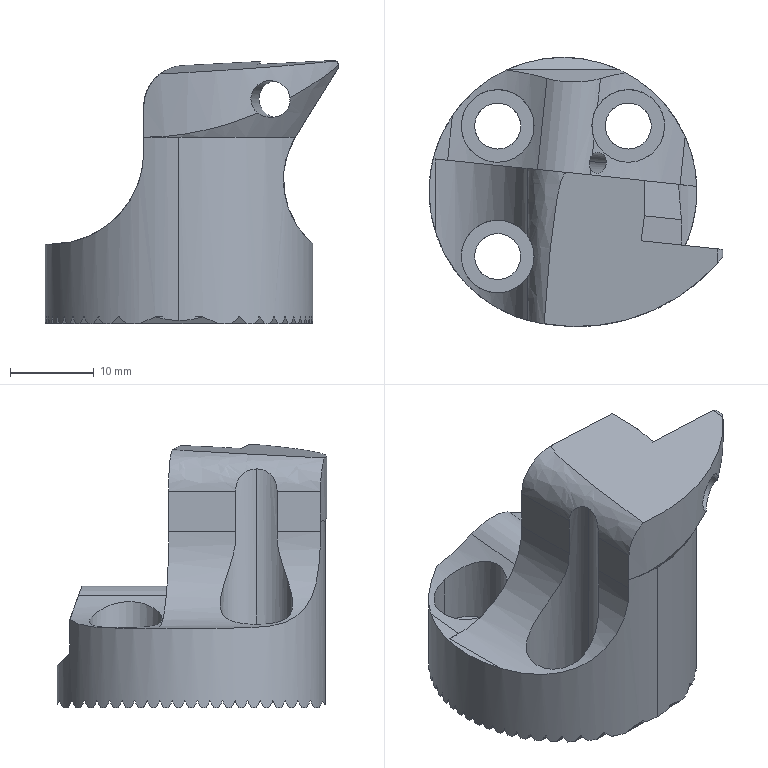NC program | Mastercam | posted with a generic post
Lines 2517 to 2597 of 7170:
(8 FEM |TOOL - 1|DIA. OFF. - 1|LEN. - 1|TOOL DIA. - 8.)
N5096 T1 M6
N5098 G0 G54 G90 X11.737 Y-6.579 C90.43 B-29.366 S3500 M3
N5100 G43 H1 Z66.467
N5102 Z17.467
N5104 G1 Z16.017 F2000.
N5106 X5.773 Y-5.92 F600.
N5108 X2.48 Y-5.556
N5110 G0 Z66.017
N5112 X11.737 Y-6.579
N5114 Z17.017
N5116 G1 Z15.567 F2000.
N5118 X5.773 Y-5.92 F600.
N5120 X2.48 Y-5.556
N5122 G0 Z65.567
N5124 X11.737 Y-6.579
N5126 Z16.567
N5128 G1 Z15.117 F2000.
N5130 X5.773 Y-5.92 F600.
N5132 X2.48 Y-5.556
N5134 G0 Z65.117
N5136 X11.737 Y-6.579
N5138 Z16.117
N5140 G1 Z14.667 F2000.
N5142 X5.773 Y-5.92 F600.
N5144 X2.48 Y-5.556
N5146 G0 Z64.667
N5148 X11.737 Y-6.579
N5150 Z15.667
N5152 G1 Z14.217 F2000.
N5154 X5.773 Y-5.92 F600.
N5156 X2.48 Y-5.556
N5158 G0 Z64.217
N5160 X11.737 Y-6.579
N5162 Z15.217
N5164 G1 Z13.767 F2000.
N5166 X5.773 Y-5.92 F600.
N5168 X2.48 Y-5.556
N5170 G0 Z63.767
N5172 X11.737 Y-6.579
N5174 Z14.767
N5176 G1 Z13.317 F2000.
N5178 X5.773 Y-5.92 F600.
N5180 X2.48 Y-5.556
N5182 G0 Z63.317
N5184 X11.737 Y-6.579
N5186 Z14.317
N5188 G1 Z12.867 F2000.
N5190 X5.773 Y-5.92 F600.
N5192 X2.48 Y-5.556
N5194 G0 Z62.867
N5196 X11.737 Y-6.579
N5198 Z13.867
N5200 G1 Z12.417 F2000.
N5202 X5.773 Y-5.92 F600.
N5204 X2.48 Y-5.556
N5206 G0 Z62.417
N5208 X11.737 Y-6.579
N5210 Z13.417
N5212 G1 Z11.967 F2000.
N5214 X5.773 Y-5.92 F600.
N5216 X2.48 Y-5.556
N5218 G0 Z66.467
N5220 M5
N5222 G0 G28 G91 Z0.
N5224 G28 C0. B0.
N5226 M01
N5228 G0 G17 G40 G80 G90 G94 G98
N5230 G0 G28 G91 Z0.
(2.5 DR |TOOL - 2|DIA. OFF. - 2|LEN. - 2|TOOL DIA. - 2.5)
N5232 T2 M6
N5234 G0 G54 G90 X4.619 Y-3.272 C90.43 B-29.366 S1500 M3
N5236 G43 H2 Z62.005
N5238 G83 G98 Z2.505 R13.005 Q2. F15.
N5240 G80
N5242 M5
N5244 G0 G28 G91 Z0.
N5246 G28 C0. B0.
N5248 M01
N5250 G0 G17 G40 G80 G90 G94 G98
N5252 G0 G28 G91 Z0.